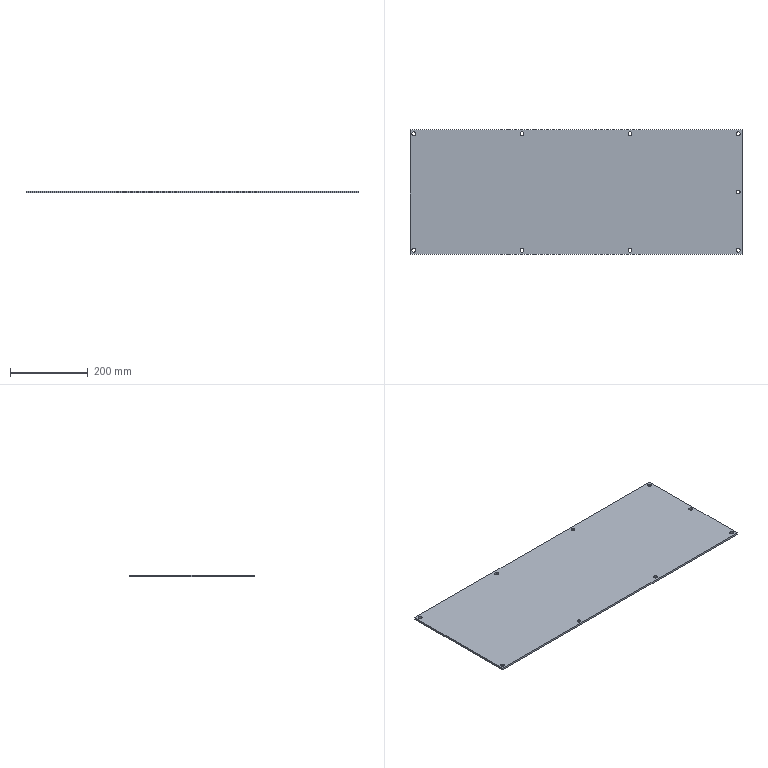Part | SolidWorks | features Extrusion 1 | 1 solid | 24 faces | box 855.022 x 319.762 x 5 mm | volume 1363482 mm3 | cylinder 18 | plane 6 | commonest cylinder face diameters 10 x18
STEP:
#1=CARTESIAN_POINT('',(840.022,159.881,5.));
#2=VERTEX_POINT('',#1);
#3=CARTESIAN_POINT('',(850.022,159.881,5.));
#4=VERTEX_POINT('',#3);
#5=CARTESIAN_POINT('',(845.022,159.881,5.));
#6=DIRECTION('',(0.,0.,1.));
#7=DIRECTION('',(1.,0.,0.));
#8=AXIS2_PLACEMENT_3D('',#5,#6,#7);
#9=CIRCLE('',#8,5.);
#10=EDGE_CURVE('',#2,#4,#9,.T.);
#11=ORIENTED_EDGE('',*,*,#10,.T.);
#12=CARTESIAN_POINT('',(850.022,159.881,0.));
#13=VERTEX_POINT('',#12);
#14=CARTESIAN_POINT('',(850.022,159.881,5.));
#15=DIRECTION('',(0.,0.,-1.));
#16=VECTOR('',#15,1000.);
#17=LINE('',#14,#16);
#18=EDGE_CURVE('',#4,#13,#17,.T.);
#19=ORIENTED_EDGE('',*,*,#18,.T.);
#20=CARTESIAN_POINT('',(840.022,159.881,0.));
#21=VERTEX_POINT('',#20);
#22=CARTESIAN_POINT('',(845.022,159.881,0.));
#23=DIRECTION('',(0.,0.,1.));
#24=DIRECTION('',(1.,0.,0.));
#25=AXIS2_PLACEMENT_3D('',#22,#23,#24);
#26=CIRCLE('',#25,5.);
#27=EDGE_CURVE('',#21,#13,#26,.T.);
#28=ORIENTED_EDGE('',*,*,#27,.F.);
#29=CARTESIAN_POINT('',(840.022,159.881,5.));
#30=DIRECTION('',(0.,0.,-1.));
#31=VECTOR('',#30,1000.);
#32=LINE('',#29,#31);
#33=EDGE_CURVE('',#2,#21,#32,.T.);
#34=ORIENTED_EDGE('',*,*,#33,.F.);
#35=EDGE_LOOP('',(#11,#19,#28,#34));
#36=FACE_OUTER_BOUND('',#35,.T.);
#37=CARTESIAN_POINT('',(845.022,159.881,5.));
#38=DIRECTION('',(0.,0.,-1.));
#39=DIRECTION('',(-1.,0.,0.));
#40=AXIS2_PLACEMENT_3D('',#37,#38,#39);
#41=CYLINDRICAL_SURFACE('',#40,5.);
#42=ADVANCED_FACE('',(#36),#41,.F.);
#43=CARTESIAN_POINT('',(561.682,10.,5.));
#44=VERTEX_POINT('',#43);
#45=CARTESIAN_POINT('',(571.682,10.,5.));
#46=VERTEX_POINT('',#45);
#47=CARTESIAN_POINT('',(566.682,10.,5.));
#48=DIRECTION('',(0.,0.,1.));
#49=DIRECTION('',(1.,0.,0.));
#50=AXIS2_PLACEMENT_3D('',#47,#48,#49);
#51=CIRCLE('',#50,5.);
#52=EDGE_CURVE('',#44,#46,#51,.T.);
#53=ORIENTED_EDGE('',*,*,#52,.T.);
#54=CARTESIAN_POINT('',(571.682,10.,0.));
#55=VERTEX_POINT('',#54);
#56=CARTESIAN_POINT('',(571.682,10.,5.));
#57=DIRECTION('',(0.,0.,-1.));
#58=VECTOR('',#57,1000.);
#59=LINE('',#56,#58);
#60=EDGE_CURVE('',#46,#55,#59,.T.);
#61=ORIENTED_EDGE('',*,*,#60,.T.);
#62=CARTESIAN_POINT('',(561.682,10.,0.));
#63=VERTEX_POINT('',#62);
#64=CARTESIAN_POINT('',(566.682,10.,0.));
#65=DIRECTION('',(0.,0.,1.));
#66=DIRECTION('',(1.,0.,0.));
#67=AXIS2_PLACEMENT_3D('',#64,#65,#66);
#68=CIRCLE('',#67,5.);
#69=EDGE_CURVE('',#63,#55,#68,.T.);
#70=ORIENTED_EDGE('',*,*,#69,.F.);
#71=CARTESIAN_POINT('',(561.682,10.,5.));
#72=DIRECTION('',(0.,0.,-1.));
#73=VECTOR('',#72,1000.);
#74=LINE('',#71,#73);
#75=EDGE_CURVE('',#44,#63,#74,.T.);
#76=ORIENTED_EDGE('',*,*,#75,.F.);
#77=EDGE_LOOP('',(#53,#61,#70,#76));
#78=FACE_OUTER_BOUND('',#77,.T.);
#79=CARTESIAN_POINT('',(566.682,10.,5.));
#80=DIRECTION('',(0.,0.,-1.));
#81=DIRECTION('',(-1.,0.,0.));
#82=AXIS2_PLACEMENT_3D('',#79,#80,#81);
#83=CYLINDRICAL_SURFACE('',#82,5.);
#84=ADVANCED_FACE('',(#78),#83,.F.);
#85=CARTESIAN_POINT('',(561.682,309.762,5.));
#86=VERTEX_POINT('',#85);
#87=CARTESIAN_POINT('',(571.682,309.762,5.));
#88=VERTEX_POINT('',#87);
#89=CARTESIAN_POINT('',(566.682,309.762,5.));
#90=DIRECTION('',(0.,0.,1.));
#91=DIRECTION('',(1.,0.,0.));
#92=AXIS2_PLACEMENT_3D('',#89,#90,#91);
#93=CIRCLE('',#92,5.);
#94=EDGE_CURVE('',#86,#88,#93,.T.);
#95=ORIENTED_EDGE('',*,*,#94,.T.);
#96=CARTESIAN_POINT('',(571.682,309.762,0.));
#97=VERTEX_POINT('',#96);
#98=CARTESIAN_POINT('',(571.682,309.762,5.));
#99=DIRECTION('',(0.,0.,-1.));
#100=VECTOR('',#99,1000.);
#101=LINE('',#98,#100);
#102=EDGE_CURVE('',#88,#97,#101,.T.);
#103=ORIENTED_EDGE('',*,*,#102,.T.);
#104=CARTESIAN_POINT('',(561.682,309.762,0.));
#105=VERTEX_POINT('',#104);
#106=CARTESIAN_POINT('',(566.682,309.762,0.));
#107=DIRECTION('',(0.,0.,1.));
#108=DIRECTION('',(1.,0.,0.));
#109=AXIS2_PLACEMENT_3D('',#106,#107,#108);
#110=CIRCLE('',#109,5.);
#111=EDGE_CURVE('',#105,#97,#110,.T.);
#112=ORIENTED_EDGE('',*,*,#111,.F.);
#113=CARTESIAN_POINT('',(561.682,309.762,5.));
#114=DIRECTION('',(0.,0.,-1.));
#115=VECTOR('',#114,1000.);
#116=LINE('',#113,#115);
#117=EDGE_CURVE('',#86,#105,#116,.T.);
#118=ORIENTED_EDGE('',*,*,#117,.F.);
#119=EDGE_LOOP('',(#95,#103,#112,#118));
#120=FACE_OUTER_BOUND('',#119,.T.);
#121=CARTESIAN_POINT('',(566.682,309.762,5.));
#122=DIRECTION('',(0.,0.,-1.));
#123=DIRECTION('',(-1.,0.,0.));
#124=AXIS2_PLACEMENT_3D('',#121,#122,#123);
#125=CYLINDRICAL_SURFACE('',#124,5.);
#126=ADVANCED_FACE('',(#120),#125,.F.);
#127=CARTESIAN_POINT('',(283.341,10.,5.));
#128=VERTEX_POINT('',#127);
#129=CARTESIAN_POINT('',(293.341,10.,5.));
#130=VERTEX_POINT('',#129);
#131=CARTESIAN_POINT('',(288.341,10.,5.));
#132=DIRECTION('',(0.,0.,1.));
#133=DIRECTION('',(1.,0.,0.));
#134=AXIS2_PLACEMENT_3D('',#131,#132,#133);
#135=CIRCLE('',#134,5.);
#136=EDGE_CURVE('',#128,#130,#135,.T.);
#137=ORIENTED_EDGE('',*,*,#136,.T.);
#138=CARTESIAN_POINT('',(293.341,10.,0.));
#139=VERTEX_POINT('',#138);
#140=CARTESIAN_POINT('',(293.341,10.,5.));
#141=DIRECTION('',(0.,0.,-1.));
#142=VECTOR('',#141,1000.);
#143=LINE('',#140,#142);
#144=EDGE_CURVE('',#130,#139,#143,.T.);
#145=ORIENTED_EDGE('',*,*,#144,.T.);
#146=CARTESIAN_POINT('',(283.341,10.,0.));
#147=VERTEX_POINT('',#146);
#148=CARTESIAN_POINT('',(288.341,10.,0.));
#149=DIRECTION('',(0.,0.,1.));
#150=DIRECTION('',(1.,0.,0.));
#151=AXIS2_PLACEMENT_3D('',#148,#149,#150);
#152=CIRCLE('',#151,5.);
#153=EDGE_CURVE('',#147,#139,#152,.T.);
#154=ORIENTED_EDGE('',*,*,#153,.F.);
#155=CARTESIAN_POINT('',(283.341,10.,5.));
#156=DIRECTION('',(0.,0.,-1.));
#157=VECTOR('',#156,1000.);
#158=LINE('',#155,#157);
#159=EDGE_CURVE('',#128,#147,#158,.T.);
#160=ORIENTED_EDGE('',*,*,#159,.F.);
#161=EDGE_LOOP('',(#137,#145,#154,#160));
#162=FACE_OUTER_BOUND('',#161,.T.);
#163=CARTESIAN_POINT('',(288.341,10.,5.));
#164=DIRECTION('',(0.,0.,-1.));
#165=DIRECTION('',(-1.,0.,0.));
#166=AXIS2_PLACEMENT_3D('',#163,#164,#165);
#167=CYLINDRICAL_SURFACE('',#166,5.);
#168=ADVANCED_FACE('',(#162),#167,.F.);
#169=CARTESIAN_POINT('',(283.341,309.762,5.));
#170=VERTEX_POINT('',#169);
#171=CARTESIAN_POINT('',(293.341,309.762,5.));
#172=VERTEX_POINT('',#171);
#173=CARTESIAN_POINT('',(288.341,309.762,5.));
#174=DIRECTION('',(0.,0.,1.));
#175=DIRECTION('',(1.,0.,0.));
#176=AXIS2_PLACEMENT_3D('',#173,#174,#175);
#177=CIRCLE('',#176,5.);
#178=EDGE_CURVE('',#170,#172,#177,.T.);
#179=ORIENTED_EDGE('',*,*,#178,.T.);
#180=CARTESIAN_POINT('',(293.341,309.762,0.));
#181=VERTEX_POINT('',#180);
#182=CARTESIAN_POINT('',(293.341,309.762,5.));
#183=DIRECTION('',(0.,0.,-1.));
#184=VECTOR('',#183,1000.);
#185=LINE('',#182,#184);
#186=EDGE_CURVE('',#172,#181,#185,.T.);
#187=ORIENTED_EDGE('',*,*,#186,.T.);
#188=CARTESIAN_POINT('',(283.341,309.762,0.));
#189=VERTEX_POINT('',#188);
#190=CARTESIAN_POINT('',(288.341,309.762,0.));
#191=DIRECTION('',(0.,0.,1.));
#192=DIRECTION('',(1.,0.,0.));
#193=AXIS2_PLACEMENT_3D('',#190,#191,#192);
#194=CIRCLE('',#193,5.);
#195=EDGE_CURVE('',#189,#181,#194,.T.);
#196=ORIENTED_EDGE('',*,*,#195,.F.);
#197=CARTESIAN_POINT('',(283.341,309.762,5.));
#198=DIRECTION('',(0.,0.,-1.));
#199=VECTOR('',#198,1000.);
#200=LINE('',#197,#199);
#201=EDGE_CURVE('',#170,#189,#200,.T.);
#202=ORIENTED_EDGE('',*,*,#201,.F.);
#203=EDGE_LOOP('',(#179,#187,#196,#202));
#204=FACE_OUTER_BOUND('',#203,.T.);
#205=CARTESIAN_POINT('',(288.341,309.762,5.));
#206=DIRECTION('',(0.,0.,-1.));
#207=DIRECTION('',(-1.,0.,0.));
#208=AXIS2_PLACEMENT_3D('',#205,#206,#207);
#209=CYLINDRICAL_SURFACE('',#208,5.);
#210=ADVANCED_FACE('',(#204),#209,.F.);
#211=CARTESIAN_POINT('',(840.022,10.,5.));
#212=VERTEX_POINT('',#211);
#213=CARTESIAN_POINT('',(850.022,10.,5.));
#214=VERTEX_POINT('',#213);
#215=CARTESIAN_POINT('',(845.022,10.,5.));
#216=DIRECTION('',(0.,0.,1.));
#217=DIRECTION('',(1.,0.,0.));
#218=AXIS2_PLACEMENT_3D('',#215,#216,#217);
#219=CIRCLE('',#218,5.);
#220=EDGE_CURVE('',#212,#214,#219,.T.);
#221=ORIENTED_EDGE('',*,*,#220,.T.);
#222=CARTESIAN_POINT('',(850.022,10.,0.));
#223=VERTEX_POINT('',#222);
#224=CARTESIAN_POINT('',(850.022,10.,5.));
#225=DIRECTION('',(0.,0.,-1.));
#226=VECTOR('',#225,1000.);
#227=LINE('',#224,#226);
#228=EDGE_CURVE('',#214,#223,#227,.T.);
#229=ORIENTED_EDGE('',*,*,#228,.T.);
#230=CARTESIAN_POINT('',(840.022,10.,0.));
#231=VERTEX_POINT('',#230);
#232=CARTESIAN_POINT('',(845.022,10.,0.));
#233=DIRECTION('',(0.,0.,1.));
#234=DIRECTION('',(1.,0.,0.));
#235=AXIS2_PLACEMENT_3D('',#232,#233,#234);
#236=CIRCLE('',#235,5.);
#237=EDGE_CURVE('',#231,#223,#236,.T.);
#238=ORIENTED_EDGE('',*,*,#237,.F.);
#239=CARTESIAN_POINT('',(840.022,10.,5.));
#240=DIRECTION('',(0.,0.,-1.));
#241=VECTOR('',#240,1000.);
#242=LINE('',#239,#241);
#243=EDGE_CURVE('',#212,#231,#242,.T.);
#244=ORIENTED_EDGE('',*,*,#243,.F.);
#245=EDGE_LOOP('',(#221,#229,#238,#244));
#246=FACE_OUTER_BOUND('',#245,.T.);
#247=CARTESIAN_POINT('',(845.022,10.,5.));
#248=DIRECTION('',(0.,0.,-1.));
#249=DIRECTION('',(-1.,0.,0.));
#250=AXIS2_PLACEMENT_3D('',#247,#248,#249);
#251=CYLINDRICAL_SURFACE('',#250,5.);
#252=ADVANCED_FACE('',(#246),#251,.F.);
#253=CARTESIAN_POINT('',(5.,10.,5.));
#254=VERTEX_POINT('',#253);
#255=CARTESIAN_POINT('',(15.,10.,5.));
#256=VERTEX_POINT('',#255);
#257=CARTESIAN_POINT('',(10.,10.,5.));
#258=DIRECTION('',(0.,0.,1.));
#259=DIRECTION('',(1.,0.,0.));
#260=AXIS2_PLACEMENT_3D('',#257,#258,#259);
#261=CIRCLE('',#260,5.);
#262=EDGE_CURVE('',#254,#256,#261,.T.);
#263=ORIENTED_EDGE('',*,*,#262,.T.);
#264=CARTESIAN_POINT('',(15.,10.,0.));
#265=VERTEX_POINT('',#264);
#266=CARTESIAN_POINT('',(15.,10.,5.));
#267=DIRECTION('',(0.,0.,-1.));
#268=VECTOR('',#267,1000.);
#269=LINE('',#266,#268);
#270=EDGE_CURVE('',#256,#265,#269,.T.);
#271=ORIENTED_EDGE('',*,*,#270,.T.);
#272=CARTESIAN_POINT('',(5.,10.,0.));
#273=VERTEX_POINT('',#272);
#274=CARTESIAN_POINT('',(10.,10.,0.));
#275=DIRECTION('',(0.,0.,1.));
#276=DIRECTION('',(1.,0.,0.));
#277=AXIS2_PLACEMENT_3D('',#274,#275,#276);
#278=CIRCLE('',#277,5.);
#279=EDGE_CURVE('',#273,#265,#278,.T.);
#280=ORIENTED_EDGE('',*,*,#279,.F.);
#281=CARTESIAN_POINT('',(5.,10.,5.));
#282=DIRECTION('',(0.,0.,-1.));
#283=VECTOR('',#282,1000.);
#284=LINE('',#281,#283);
#285=EDGE_CURVE('',#254,#273,#284,.T.);
#286=ORIENTED_EDGE('',*,*,#285,.F.);
#287=EDGE_LOOP('',(#263,#271,#280,#286));
#288=FACE_OUTER_BOUND('',#287,.T.);
#289=CARTESIAN_POINT('',(10.,10.,5.));
#290=DIRECTION('',(0.,0.,-1.));
#291=DIRECTION('',(-1.,0.,0.));
#292=AXIS2_PLACEMENT_3D('',#289,#290,#291);
#293=CYLINDRICAL_SURFACE('',#292,5.);
#294=ADVANCED_FACE('',(#288),#293,.F.);
#295=CARTESIAN_POINT('',(840.022,309.762,5.));
#296=VERTEX_POINT('',#295);
#297=CARTESIAN_POINT('',(850.022,309.762,5.));
#298=VERTEX_POINT('',#297);
#299=CARTESIAN_POINT('',(845.022,309.762,5.));
#300=DIRECTION('',(0.,0.,1.));
#301=DIRECTION('',(1.,0.,0.));
#302=AXIS2_PLACEMENT_3D('',#299,#300,#301);
#303=CIRCLE('',#302,5.);
#304=EDGE_CURVE('',#296,#298,#303,.T.);
#305=ORIENTED_EDGE('',*,*,#304,.T.);
#306=CARTESIAN_POINT('',(850.022,309.762,0.));
#307=VERTEX_POINT('',#306);
#308=CARTESIAN_POINT('',(850.022,309.762,5.));
#309=DIRECTION('',(0.,0.,-1.));
#310=VECTOR('',#309,1000.);
#311=LINE('',#308,#310);
#312=EDGE_CURVE('',#298,#307,#311,.T.);
#313=ORIENTED_EDGE('',*,*,#312,.T.);
#314=CARTESIAN_POINT('',(840.022,309.762,0.));
#315=VERTEX_POINT('',#314);
#316=CARTESIAN_POINT('',(845.022,309.762,0.));
#317=DIRECTION('',(0.,0.,1.));
#318=DIRECTION('',(1.,0.,0.));
#319=AXIS2_PLACEMENT_3D('',#316,#317,#318);
#320=CIRCLE('',#319,5.);
#321=EDGE_CURVE('',#315,#307,#320,.T.);
#322=ORIENTED_EDGE('',*,*,#321,.F.);
#323=CARTESIAN_POINT('',(840.022,309.762,5.));
#324=DIRECTION('',(0.,0.,-1.));
#325=VECTOR('',#324,1000.);
#326=LINE('',#323,#325);
#327=EDGE_CURVE('',#296,#315,#326,.T.);
#328=ORIENTED_EDGE('',*,*,#327,.F.);
#329=EDGE_LOOP('',(#305,#313,#322,#328));
#330=FACE_OUTER_BOUND('',#329,.T.);
#331=CARTESIAN_POINT('',(845.022,309.762,5.));
#332=DIRECTION('',(0.,0.,-1.));
#333=DIRECTION('',(-1.,0.,0.));
#334=AXIS2_PLACEMENT_3D('',#331,#332,#333);
#335=CYLINDRICAL_SURFACE('',#334,5.);
#336=ADVANCED_FACE('',(#330),#335,.F.);
#337=CARTESIAN_POINT('',(5.,309.762,5.));
#338=VERTEX_POINT('',#337);
#339=CARTESIAN_POINT('',(15.,309.762,5.));
#340=VERTEX_POINT('',#339);
#341=CARTESIAN_POINT('',(10.,309.762,5.));
#342=DIRECTION('',(0.,0.,1.));
#343=DIRECTION('',(1.,0.,0.));
#344=AXIS2_PLACEMENT_3D('',#341,#342,#343);
#345=CIRCLE('',#344,5.);
#346=EDGE_CURVE('',#338,#340,#345,.T.);
#347=ORIENTED_EDGE('',*,*,#346,.T.);
#348=CARTESIAN_POINT('',(15.,309.762,0.));
#349=VERTEX_POINT('',#348);
#350=CARTESIAN_POINT('',(15.,309.762,5.));
#351=DIRECTION('',(0.,0.,-1.));
#352=VECTOR('',#351,1000.);
#353=LINE('',#350,#352);
#354=EDGE_CURVE('',#340,#349,#353,.T.);
#355=ORIENTED_EDGE('',*,*,#354,.T.);
#356=CARTESIAN_POINT('',(5.,309.762,0.));
#357=VERTEX_POINT('',#356);
#358=CARTESIAN_POINT('',(10.,309.762,0.));
#359=DIRECTION('',(0.,0.,1.));
#360=DIRECTION('',(1.,0.,0.));
#361=AXIS2_PLACEMENT_3D('',#358,#359,#360);
#362=CIRCLE('',#361,5.);
#363=EDGE_CURVE('',#357,#349,#362,.T.);
#364=ORIENTED_EDGE('',*,*,#363,.F.);
#365=CARTESIAN_POINT('',(5.,309.762,5.));
#366=DIRECTION('',(0.,0.,-1.));
#367=VECTOR('',#366,1000.);
#368=LINE('',#365,#367);
#369=EDGE_CURVE('',#338,#357,#368,.T.);
#370=ORIENTED_EDGE('',*,*,#369,.F.);
#371=EDGE_LOOP('',(#347,#355,#364,#370));
#372=FACE_OUTER_BOUND('',#371,.T.);
#373=CARTESIAN_POINT('',(10.,309.762,5.));
#374=DIRECTION('',(0.,0.,-1.));
#375=DIRECTION('',(-1.,0.,0.));
#376=AXIS2_PLACEMENT_3D('',#373,#374,#375);
#377=CYLINDRICAL_SURFACE('',#376,5.);
#378=ADVANCED_FACE('',(#372),#377,.F.);
#379=CARTESIAN_POINT('',(0.,319.762,5.));
#380=VERTEX_POINT('',#379);
#381=CARTESIAN_POINT('',(0.,0.,5.));
#382=VERTEX_POINT('',#381);
#383=CARTESIAN_POINT('',(0.,0.,5.));
#384=DIRECTION('',(0.,-1.,0.));
#385=VECTOR('',#384,1000.);
#386=LINE('',#383,#385);
#387=EDGE_CURVE('',#380,#382,#386,.T.);
#388=ORIENTED_EDGE('',*,*,#387,.T.);
#389=CARTESIAN_POINT('',(855.022,0.,5.));
#390=VERTEX_POINT('',#389);
#391=CARTESIAN_POINT('',(855.022,0.,5.));
#392=DIRECTION('',(1.,0.,0.));
#393=VECTOR('',#392,1000.);
#394=LINE('',#391,#393);
#395=EDGE_CURVE('',#382,#390,#394,.T.);
#396=ORIENTED_EDGE('',*,*,#395,.T.);
#397=CARTESIAN_POINT('',(855.022,319.762,5.));
#398=VERTEX_POINT('',#397);
#399=CARTESIAN_POINT('',(855.022,319.762,5.));
#400=DIRECTION('',(0.,1.,0.));
#401=VECTOR('',#400,1000.);
#402=LINE('',#399,#401);
#403=EDGE_CURVE('',#390,#398,#402,.T.);
#404=ORIENTED_EDGE('',*,*,#403,.T.);
#405=CARTESIAN_POINT('',(0.,319.762,5.));
#406=DIRECTION('',(-1.,0.,0.));
#407=VECTOR('',#406,1000.);
#408=LINE('',#405,#407);
#409=EDGE_CURVE('',#398,#380,#408,.T.);
#410=ORIENTED_EDGE('',*,*,#409,.T.);
#411=EDGE_LOOP('',(#388,#396,#404,#410));
#412=FACE_OUTER_BOUND('',#411,.T.);
#413=ORIENTED_EDGE('',*,*,#346,.F.);
#414=CARTESIAN_POINT('',(10.,309.762,5.));
#415=DIRECTION('',(0.,0.,1.));
#416=DIRECTION('',(1.,0.,0.));
#417=AXIS2_PLACEMENT_3D('',#414,#415,#416);
#418=CIRCLE('',#417,5.);
#419=EDGE_CURVE('',#340,#338,#418,.T.);
#420=ORIENTED_EDGE('',*,*,#419,.F.);
#421=EDGE_LOOP('',(#413,#420));
#422=FACE_BOUND('',#421,.T.);
#423=ORIENTED_EDGE('',*,*,#304,.F.);
#424=CARTESIAN_POINT('',(845.022,309.762,5.));
#425=DIRECTION('',(0.,0.,1.));
#426=DIRECTION('',(1.,0.,0.));
#427=AXIS2_PLACEMENT_3D('',#424,#425,#426);
#428=CIRCLE('',#427,5.);
#429=EDGE_CURVE('',#298,#296,#428,.T.);
#430=ORIENTED_EDGE('',*,*,#429,.F.);
#431=EDGE_LOOP('',(#423,#430));
#432=FACE_BOUND('',#431,.T.);
#433=ORIENTED_EDGE('',*,*,#262,.F.);
#434=CARTESIAN_POINT('',(10.,10.,5.));
#435=DIRECTION('',(0.,0.,1.));
#436=DIRECTION('',(1.,0.,0.));
#437=AXIS2_PLACEMENT_3D('',#434,#435,#436);
#438=CIRCLE('',#437,5.);
#439=EDGE_CURVE('',#256,#254,#438,.T.);
#440=ORIENTED_EDGE('',*,*,#439,.F.);
#441=EDGE_LOOP('',(#433,#440));
#442=FACE_BOUND('',#441,.T.);
#443=ORIENTED_EDGE('',*,*,#220,.F.);
#444=CARTESIAN_POINT('',(845.022,10.,5.));
#445=DIRECTION('',(0.,0.,1.));
#446=DIRECTION('',(1.,0.,0.));
#447=AXIS2_PLACEMENT_3D('',#444,#445,#446);
#448=CIRCLE('',#447,5.);
#449=EDGE_CURVE('',#214,#212,#448,.T.);
#450=ORIENTED_EDGE('',*,*,#449,.F.);
#451=EDGE_LOOP('',(#443,#450));
#452=FACE_BOUND('',#451,.T.);
#453=ORIENTED_EDGE('',*,*,#178,.F.);
#454=CARTESIAN_POINT('',(288.341,309.762,5.));
#455=DIRECTION('',(0.,0.,1.));
#456=DIRECTION('',(1.,0.,0.));
#457=AXIS2_PLACEMENT_3D('',#454,#455,#456);
#458=CIRCLE('',#457,5.);
#459=EDGE_CURVE('',#172,#170,#458,.T.);
#460=ORIENTED_EDGE('',*,*,#459,.F.);
#461=EDGE_LOOP('',(#453,#460));
#462=FACE_BOUND('',#461,.T.);
#463=ORIENTED_EDGE('',*,*,#136,.F.);
#464=CARTESIAN_POINT('',(288.341,10.,5.));
#465=DIRECTION('',(0.,0.,1.));
#466=DIRECTION('',(1.,0.,0.));
#467=AXIS2_PLACEMENT_3D('',#464,#465,#466);
#468=CIRCLE('',#467,5.);
#469=EDGE_CURVE('',#130,#128,#468,.T.);
#470=ORIENTED_EDGE('',*,*,#469,.F.);
#471=EDGE_LOOP('',(#463,#470));
#472=FACE_BOUND('',#471,.T.);
#473=ORIENTED_EDGE('',*,*,#94,.F.);
#474=CARTESIAN_POINT('',(566.682,309.762,5.));
#475=DIRECTION('',(0.,0.,1.));
#476=DIRECTION('',(1.,0.,0.));
#477=AXIS2_PLACEMENT_3D('',#474,#475,#476);
#478=CIRCLE('',#477,5.);
#479=EDGE_CURVE('',#88,#86,#478,.T.);
#480=ORIENTED_EDGE('',*,*,#479,.F.);
#481=EDGE_LOOP('',(#473,#480));
#482=FACE_BOUND('',#481,.T.);
#483=ORIENTED_EDGE('',*,*,#52,.F.);
#484=CARTESIAN_POINT('',(566.682,10.,5.));
#485=DIRECTION('',(0.,0.,1.));
#486=DIRECTION('',(1.,0.,0.));
#487=AXIS2_PLACEMENT_3D('',#484,#485,#486);
#488=CIRCLE('',#487,5.);
#489=EDGE_CURVE('',#46,#44,#488,.T.);
#490=ORIENTED_EDGE('',*,*,#489,.F.);
#491=EDGE_LOOP('',(#483,#490));
#492=FACE_BOUND('',#491,.T.);
#493=ORIENTED_EDGE('',*,*,#10,.F.);
#494=CARTESIAN_POINT('',(845.022,159.881,5.));
#495=DIRECTION('',(0.,0.,1.));
#496=DIRECTION('',(1.,0.,0.));
#497=AXIS2_PLACEMENT_3D('',#494,#495,#496);
#498=CIRCLE('',#497,5.);
#499=EDGE_CURVE('',#4,#2,#498,.T.);
#500=ORIENTED_EDGE('',*,*,#499,.F.);
#501=EDGE_LOOP('',(#493,#500));
#502=FACE_BOUND('',#501,.T.);
#503=CARTESIAN_POINT('',(0.,0.,5.));
#504=DIRECTION('',(0.,0.,-1.));
#505=DIRECTION('',(-1.,0.,0.));
#506=AXIS2_PLACEMENT_3D('',#503,#504,#505);
#507=PLANE('',#506);
#508=ADVANCED_FACE('',(#412,#422,#432,#442,#452,#462,#472,#482,#492,#502),#507,.F.);
#509=ORIENTED_EDGE('',*,*,#69,.T.);
#510=CARTESIAN_POINT('',(566.682,10.,0.));
#511=DIRECTION('',(0.,0.,1.));
#512=DIRECTION('',(1.,0.,0.));
#513=AXIS2_PLACEMENT_3D('',#510,#511,#512);
#514=CIRCLE('',#513,5.);
#515=EDGE_CURVE('',#55,#63,#514,.T.);
#516=ORIENTED_EDGE('',*,*,#515,.T.);
#517=EDGE_LOOP('',(#509,#516));
#518=FACE_BOUND('',#517,.T.);
#519=ORIENTED_EDGE('',*,*,#153,.T.);
#520=CARTESIAN_POINT('',(288.341,10.,0.));
#521=DIRECTION('',(0.,0.,1.));
#522=DIRECTION('',(1.,0.,0.));
#523=AXIS2_PLACEMENT_3D('',#520,#521,#522);
#524=CIRCLE('',#523,5.);
#525=EDGE_CURVE('',#139,#147,#524,.T.);
#526=ORIENTED_EDGE('',*,*,#525,.T.);
#527=EDGE_LOOP('',(#519,#526));
#528=FACE_BOUND('',#527,.T.);
#529=ORIENTED_EDGE('',*,*,#237,.T.);
#530=CARTESIAN_POINT('',(845.022,10.,0.));
#531=DIRECTION('',(0.,0.,1.));
#532=DIRECTION('',(1.,0.,0.));
#533=AXIS2_PLACEMENT_3D('',#530,#531,#532);
#534=CIRCLE('',#533,5.);
#535=EDGE_CURVE('',#223,#231,#534,.T.);
#536=ORIENTED_EDGE('',*,*,#535,.T.);
#537=EDGE_LOOP('',(#529,#536));
#538=FACE_BOUND('',#537,.T.);
#539=ORIENTED_EDGE('',*,*,#321,.T.);
#540=CARTESIAN_POINT('',(845.022,309.762,0.));
#541=DIRECTION('',(0.,0.,1.));
#542=DIRECTION('',(1.,0.,0.));
#543=AXIS2_PLACEMENT_3D('',#540,#541,#542);
#544=CIRCLE('',#543,5.);
#545=EDGE_CURVE('',#307,#315,#544,.T.);
#546=ORIENTED_EDGE('',*,*,#545,.T.);
#547=EDGE_LOOP('',(#539,#546));
#548=FACE_BOUND('',#547,.T.);
#549=CARTESIAN_POINT('',(0.,319.762,0.));
#550=VERTEX_POINT('',#549);
#551=CARTESIAN_POINT('',(0.,0.,0.));
#552=VERTEX_POINT('',#551);
#553=CARTESIAN_POINT('',(0.,0.,0.));
#554=DIRECTION('',(0.,-1.,0.));
#555=VECTOR('',#554,1000.);
#556=LINE('',#553,#555);
#557=EDGE_CURVE('',#550,#552,#556,.T.);
#558=ORIENTED_EDGE('',*,*,#557,.F.);
#559=CARTESIAN_POINT('',(855.022,319.762,0.));
#560=VERTEX_POINT('',#559);
#561=CARTESIAN_POINT('',(0.,319.762,0.));
#562=DIRECTION('',(-1.,0.,0.));
#563=VECTOR('',#562,1000.);
#564=LINE('',#561,#563);
#565=EDGE_CURVE('',#560,#550,#564,.T.);
#566=ORIENTED_EDGE('',*,*,#565,.F.);
#567=CARTESIAN_POINT('',(855.022,0.,0.));
#568=VERTEX_POINT('',#567);
#569=CARTESIAN_POINT('',(855.022,319.762,0.));
#570=DIRECTION('',(0.,1.,0.));
#571=VECTOR('',#570,1000.);
#572=LINE('',#569,#571);
#573=EDGE_CURVE('',#568,#560,#572,.T.);
#574=ORIENTED_EDGE('',*,*,#573,.F.);
#575=CARTESIAN_POINT('',(855.022,0.,0.));
#576=DIRECTION('',(1.,0.,0.));
#577=VECTOR('',#576,1000.);
#578=LINE('',#575,#577);
#579=EDGE_CURVE('',#552,#568,#578,.T.);
#580=ORIENTED_EDGE('',*,*,#579,.F.);
#581=EDGE_LOOP('',(#558,#566,#574,#580));
#582=FACE_OUTER_BOUND('',#581,.T.);
#583=ORIENTED_EDGE('',*,*,#363,.T.);
#584=CARTESIAN_POINT('',(10.,309.762,0.));
#585=DIRECTION('',(0.,0.,1.));
#586=DIRECTION('',(1.,0.,0.));
#587=AXIS2_PLACEMENT_3D('',#584,#585,#586);
#588=CIRCLE('',#587,5.);
#589=EDGE_CURVE('',#349,#357,#588,.T.);
#590=ORIENTED_EDGE('',*,*,#589,.T.);
#591=EDGE_LOOP('',(#583,#590));
#592=FACE_BOUND('',#591,.T.);
#593=ORIENTED_EDGE('',*,*,#279,.T.);
#594=CARTESIAN_POINT('',(10.,10.,0.));
#595=DIRECTION('',(0.,0.,1.));
#596=DIRECTION('',(1.,0.,0.));
#597=AXIS2_PLACEMENT_3D('',#594,#595,#596);
#598=CIRCLE('',#597,5.);
#599=EDGE_CURVE('',#265,#273,#598,.T.);
#600=ORIENTED_EDGE('',*,*,#599,.T.);
#601=EDGE_LOOP('',(#593,#600));
#602=FACE_BOUND('',#601,.T.);
#603=ORIENTED_EDGE('',*,*,#195,.T.);
#604=CARTESIAN_POINT('',(288.341,309.762,0.));
#605=DIRECTION('',(0.,0.,1.));
#606=DIRECTION('',(1.,0.,0.));
#607=AXIS2_PLACEMENT_3D('',#604,#605,#606);
#608=CIRCLE('',#607,5.);
#609=EDGE_CURVE('',#181,#189,#608,.T.);
#610=ORIENTED_EDGE('',*,*,#609,.T.);
#611=EDGE_LOOP('',(#603,#610));
#612=FACE_BOUND('',#611,.T.);
#613=ORIENTED_EDGE('',*,*,#111,.T.);
#614=CARTESIAN_POINT('',(566.682,309.762,0.));
#615=DIRECTION('',(0.,0.,1.));
#616=DIRECTION('',(1.,0.,0.));
#617=AXIS2_PLACEMENT_3D('',#614,#615,#616);
#618=CIRCLE('',#617,5.);
#619=EDGE_CURVE('',#97,#105,#618,.T.);
#620=ORIENTED_EDGE('',*,*,#619,.T.);
#621=EDGE_LOOP('',(#613,#620));
#622=FACE_BOUND('',#621,.T.);
#623=ORIENTED_EDGE('',*,*,#27,.T.);
#624=CARTESIAN_POINT('',(845.022,159.881,0.));
#625=DIRECTION('',(0.,0.,1.));
#626=DIRECTION('',(1.,0.,0.));
#627=AXIS2_PLACEMENT_3D('',#624,#625,#626);
#628=CIRCLE('',#627,5.);
#629=EDGE_CURVE('',#13,#21,#628,.T.);
#630=ORIENTED_EDGE('',*,*,#629,.T.);
#631=EDGE_LOOP('',(#623,#630));
#632=FACE_BOUND('',#631,.T.);
#633=CARTESIAN_POINT('',(0.,0.,0.));
#634=DIRECTION('',(0.,0.,-1.));
#635=DIRECTION('',(-1.,0.,0.));
#636=AXIS2_PLACEMENT_3D('',#633,#634,#635);
#637=PLANE('',#636);
#638=ADVANCED_FACE('',(#518,#528,#538,#548,#582,#592,#602,#612,#622,#632),#637,.T.);
#639=ORIENTED_EDGE('',*,*,#557,.T.);
#640=CARTESIAN_POINT('',(0.,0.,5.));
#641=DIRECTION('',(0.,0.,-1.));
#642=VECTOR('',#641,1000.);
#643=LINE('',#640,#642);
#644=EDGE_CURVE('',#382,#552,#643,.T.);
#645=ORIENTED_EDGE('',*,*,#644,.F.);
#646=ORIENTED_EDGE('',*,*,#387,.F.);
#647=CARTESIAN_POINT('',(0.,319.762,5.));
#648=DIRECTION('',(0.,0.,-1.));
#649=VECTOR('',#648,1000.);
#650=LINE('',#647,#649);
#651=EDGE_CURVE('',#380,#550,#650,.T.);
#652=ORIENTED_EDGE('',*,*,#651,.T.);
#653=EDGE_LOOP('',(#639,#645,#646,#652));
#654=FACE_OUTER_BOUND('',#653,.T.);
#655=CARTESIAN_POINT('',(0.,0.,5.));
#656=DIRECTION('',(1.,0.,0.));
#657=DIRECTION('',(0.,0.,-1.));
#658=AXIS2_PLACEMENT_3D('',#655,#656,#657);
#659=PLANE('',#658);
#660=ADVANCED_FACE('',(#654),#659,.F.);
#661=ORIENTED_EDGE('',*,*,#579,.T.);
#662=CARTESIAN_POINT('',(855.022,0.,5.));
#663=DIRECTION('',(0.,0.,-1.));
#664=VECTOR('',#663,1000.);
#665=LINE('',#662,#664);
#666=EDGE_CURVE('',#390,#568,#665,.T.);
#667=ORIENTED_EDGE('',*,*,#666,.F.);
#668=ORIENTED_EDGE('',*,*,#395,.F.);
#669=ORIENTED_EDGE('',*,*,#644,.T.);
#670=EDGE_LOOP('',(#661,#667,#668,#669));
#671=FACE_OUTER_BOUND('',#670,.T.);
#672=CARTESIAN_POINT('',(855.022,0.,5.));
#673=DIRECTION('',(0.,1.,0.));
#674=DIRECTION('',(0.,0.,1.));
#675=AXIS2_PLACEMENT_3D('',#672,#673,#674);
#676=PLANE('',#675);
#677=ADVANCED_FACE('',(#671),#676,.F.);
#678=ORIENTED_EDGE('',*,*,#573,.T.);
#679=CARTESIAN_POINT('',(855.022,319.762,5.));
#680=DIRECTION('',(0.,0.,-1.));
#681=VECTOR('',#680,1000.);
#682=LINE('',#679,#681);
#683=EDGE_CURVE('',#398,#560,#682,.T.);
#684=ORIENTED_EDGE('',*,*,#683,.F.);
#685=ORIENTED_EDGE('',*,*,#403,.F.);
#686=ORIENTED_EDGE('',*,*,#666,.T.);
#687=EDGE_LOOP('',(#678,#684,#685,#686));
#688=FACE_OUTER_BOUND('',#687,.T.);
#689=CARTESIAN_POINT('',(855.022,319.762,5.));
#690=DIRECTION('',(-1.,0.,0.));
#691=DIRECTION('',(0.,0.,1.));
#692=AXIS2_PLACEMENT_3D('',#689,#690,#691);
#693=PLANE('',#692);
#694=ADVANCED_FACE('',(#688),#693,.F.);
#695=ORIENTED_EDGE('',*,*,#565,.T.);
#696=ORIENTED_EDGE('',*,*,#651,.F.);
#697=ORIENTED_EDGE('',*,*,#409,.F.);
#698=ORIENTED_EDGE('',*,*,#683,.T.);
#699=EDGE_LOOP('',(#695,#696,#697,#698));
#700=FACE_OUTER_BOUND('',#699,.T.);
#701=CARTESIAN_POINT('',(0.,319.762,5.));
#702=DIRECTION('',(0.,-1.,0.));
#703=DIRECTION('',(0.,0.,-1.));
#704=AXIS2_PLACEMENT_3D('',#701,#702,#703);
#705=PLANE('',#704);
#706=ADVANCED_FACE('',(#700),#705,.F.);
#707=ORIENTED_EDGE('',*,*,#354,.F.);
#708=ORIENTED_EDGE('',*,*,#419,.T.);
#709=ORIENTED_EDGE('',*,*,#369,.T.);
#710=ORIENTED_EDGE('',*,*,#589,.F.);
#711=EDGE_LOOP('',(#707,#708,#709,#710));
#712=FACE_OUTER_BOUND('',#711,.T.);
#713=CARTESIAN_POINT('',(10.,309.762,5.));
#714=DIRECTION('',(0.,0.,-1.));
#715=DIRECTION('',(-1.,0.,0.));
#716=AXIS2_PLACEMENT_3D('',#713,#714,#715);
#717=CYLINDRICAL_SURFACE('',#716,5.);
#718=ADVANCED_FACE('',(#712),#717,.F.);
#719=ORIENTED_EDGE('',*,*,#312,.F.);
#720=ORIENTED_EDGE('',*,*,#429,.T.);
#721=ORIENTED_EDGE('',*,*,#327,.T.);
#722=ORIENTED_EDGE('',*,*,#545,.F.);
#723=EDGE_LOOP('',(#719,#720,#721,#722));
#724=FACE_OUTER_BOUND('',#723,.T.);
#725=CARTESIAN_POINT('',(845.022,309.762,5.));
#726=DIRECTION('',(0.,0.,-1.));
#727=DIRECTION('',(-1.,0.,0.));
#728=AXIS2_PLACEMENT_3D('',#725,#726,#727);
#729=CYLINDRICAL_SURFACE('',#728,5.);
#730=ADVANCED_FACE('',(#724),#729,.F.);
#731=ORIENTED_EDGE('',*,*,#270,.F.);
#732=ORIENTED_EDGE('',*,*,#439,.T.);
#733=ORIENTED_EDGE('',*,*,#285,.T.);
#734=ORIENTED_EDGE('',*,*,#599,.F.);
#735=EDGE_LOOP('',(#731,#732,#733,#734));
#736=FACE_OUTER_BOUND('',#735,.T.);
#737=CARTESIAN_POINT('',(10.,10.,5.));
#738=DIRECTION('',(0.,0.,-1.));
#739=DIRECTION('',(-1.,0.,0.));
#740=AXIS2_PLACEMENT_3D('',#737,#738,#739);
#741=CYLINDRICAL_SURFACE('',#740,5.);
#742=ADVANCED_FACE('',(#736),#741,.F.);
#743=ORIENTED_EDGE('',*,*,#228,.F.);
#744=ORIENTED_EDGE('',*,*,#449,.T.);
#745=ORIENTED_EDGE('',*,*,#243,.T.);
#746=ORIENTED_EDGE('',*,*,#535,.F.);
#747=EDGE_LOOP('',(#743,#744,#745,#746));
#748=FACE_OUTER_BOUND('',#747,.T.);
#749=CARTESIAN_POINT('',(845.022,10.,5.));
#750=DIRECTION('',(0.,0.,-1.));
#751=DIRECTION('',(-1.,0.,0.));
#752=AXIS2_PLACEMENT_3D('',#749,#750,#751);
#753=CYLINDRICAL_SURFACE('',#752,5.);
#754=ADVANCED_FACE('',(#748),#753,.F.);
#755=ORIENTED_EDGE('',*,*,#186,.F.);
#756=ORIENTED_EDGE('',*,*,#459,.T.);
#757=ORIENTED_EDGE('',*,*,#201,.T.);
#758=ORIENTED_EDGE('',*,*,#609,.F.);
#759=EDGE_LOOP('',(#755,#756,#757,#758));
#760=FACE_OUTER_BOUND('',#759,.T.);
#761=CARTESIAN_POINT('',(288.341,309.762,5.));
#762=DIRECTION('',(0.,0.,-1.));
#763=DIRECTION('',(-1.,0.,0.));
#764=AXIS2_PLACEMENT_3D('',#761,#762,#763);
#765=CYLINDRICAL_SURFACE('',#764,5.);
#766=ADVANCED_FACE('',(#760),#765,.F.);
#767=ORIENTED_EDGE('',*,*,#144,.F.);
#768=ORIENTED_EDGE('',*,*,#469,.T.);
#769=ORIENTED_EDGE('',*,*,#159,.T.);
#770=ORIENTED_EDGE('',*,*,#525,.F.);
#771=EDGE_LOOP('',(#767,#768,#769,#770));
#772=FACE_OUTER_BOUND('',#771,.T.);
#773=CARTESIAN_POINT('',(288.341,10.,5.));
#774=DIRECTION('',(0.,0.,-1.));
#775=DIRECTION('',(-1.,0.,0.));
#776=AXIS2_PLACEMENT_3D('',#773,#774,#775);
#777=CYLINDRICAL_SURFACE('',#776,5.);
#778=ADVANCED_FACE('',(#772),#777,.F.);
#779=ORIENTED_EDGE('',*,*,#102,.F.);
#780=ORIENTED_EDGE('',*,*,#479,.T.);
#781=ORIENTED_EDGE('',*,*,#117,.T.);
#782=ORIENTED_EDGE('',*,*,#619,.F.);
#783=EDGE_LOOP('',(#779,#780,#781,#782));
#784=FACE_OUTER_BOUND('',#783,.T.);
#785=CARTESIAN_POINT('',(566.682,309.762,5.));
#786=DIRECTION('',(0.,0.,-1.));
#787=DIRECTION('',(-1.,0.,0.));
#788=AXIS2_PLACEMENT_3D('',#785,#786,#787);
#789=CYLINDRICAL_SURFACE('',#788,5.);
#790=ADVANCED_FACE('',(#784),#789,.F.);
#791=ORIENTED_EDGE('',*,*,#60,.F.);
#792=ORIENTED_EDGE('',*,*,#489,.T.);
#793=ORIENTED_EDGE('',*,*,#75,.T.);
#794=ORIENTED_EDGE('',*,*,#515,.F.);
#795=EDGE_LOOP('',(#791,#792,#793,#794));
#796=FACE_OUTER_BOUND('',#795,.T.);
#797=CARTESIAN_POINT('',(566.682,10.,5.));
#798=DIRECTION('',(0.,0.,-1.));
#799=DIRECTION('',(-1.,0.,0.));
#800=AXIS2_PLACEMENT_3D('',#797,#798,#799);
#801=CYLINDRICAL_SURFACE('',#800,5.);
#802=ADVANCED_FACE('',(#796),#801,.F.);
#803=ORIENTED_EDGE('',*,*,#18,.F.);
#804=ORIENTED_EDGE('',*,*,#499,.T.);
#805=ORIENTED_EDGE('',*,*,#33,.T.);
#806=ORIENTED_EDGE('',*,*,#629,.F.);
#807=EDGE_LOOP('',(#803,#804,#805,#806));
#808=FACE_OUTER_BOUND('',#807,.T.);
#809=CARTESIAN_POINT('',(845.022,159.881,5.));
#810=DIRECTION('',(0.,0.,-1.));
#811=DIRECTION('',(-1.,0.,0.));
#812=AXIS2_PLACEMENT_3D('',#809,#810,#811);
#813=CYLINDRICAL_SURFACE('',#812,5.);
#814=ADVANCED_FACE('',(#808),#813,.F.);
#815=CLOSED_SHELL('',(#42,#84,#126,#168,#210,#252,#294,#336,#378,#508,#638,#660,#677,#694,#706,#718,#730,#742,#754,#766,#778,#790,#802,#814));
#816=MANIFOLD_SOLID_BREP('',#815);
#817=CARTESIAN_POINT('',(0.,0.,0.));
#818=DIRECTION('',(0.,0.,1.));
#819=DIRECTION('',(1.,0.,0.));
#820=AXIS2_PLACEMENT_3D('',#817,#818,#819);
#821=(LENGTH_UNIT()NAMED_UNIT(*)SI_UNIT(.MILLI.,.METRE.));
#822=UNCERTAINTY_MEASURE_WITH_UNIT(LENGTH_MEASURE(0.00001),#821,'','');
#823=(NAMED_UNIT(*)PLANE_ANGLE_UNIT()SI_UNIT($,.RADIAN.));
#824=(NAMED_UNIT(*)SI_UNIT($,.STERADIAN.)SOLID_ANGLE_UNIT());
#825=(GEOMETRIC_REPRESENTATION_CONTEXT(3)GLOBAL_UNCERTAINTY_ASSIGNED_CONTEXT((#822))GLOBAL_UNIT_ASSIGNED_CONTEXT((#821,#823,#824))REPRESENTATION_CONTEXT('',''));
#826=ADVANCED_BREP_SHAPE_REPRESENTATION('',(#816,#820),#825);